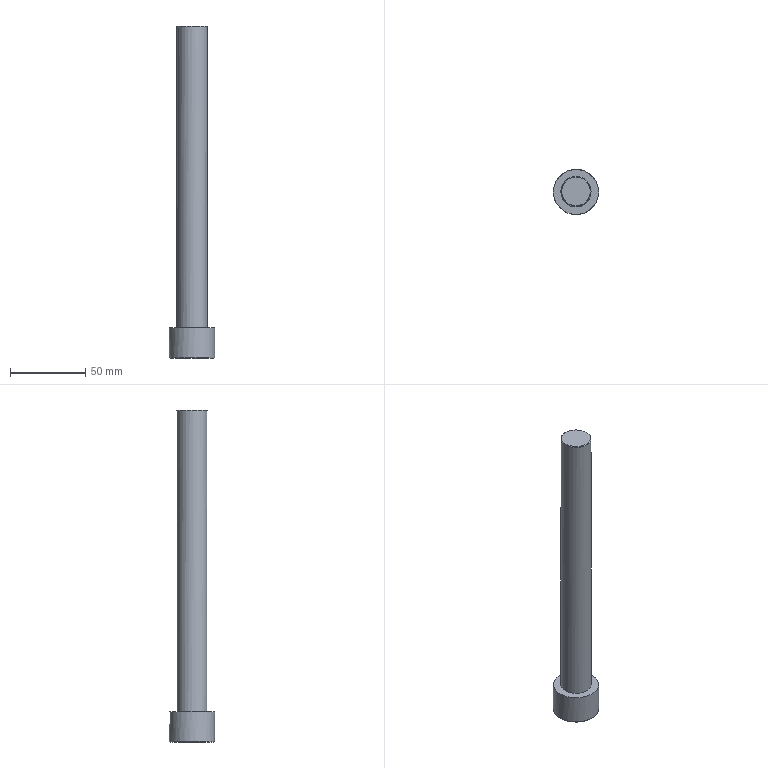Part | NX | features 模具.stp<1>[29] 2 | 1 solid | 14 faces | box 30 x 30 x 220 mm | volume 74453 mm3 | plane 10 | cylinder 2 | cone 1 | torus 1 | commonest cylinder face diameters 20 x1 30 x1
STEP:
#1=CARTESIAN_POINT('',(259.815,225.,-274.5));
#2=VERTEX_POINT('',#1);
#3=CARTESIAN_POINT('',(254.907,216.5,-274.5));
#4=VERTEX_POINT('',#3);
#5=CARTESIAN_POINT('',(259.815,225.,-274.5));
#6=DIRECTION('',(-0.5,-0.866,0.));
#7=VECTOR('',#6,1000.);
#8=LINE('',#5,#7);
#9=EDGE_CURVE('',#2,#4,#8,.T.);
#10=ORIENTED_EDGE('',*,*,#9,.T.);
#11=CARTESIAN_POINT('',(245.093,216.5,-274.5));
#12=VERTEX_POINT('',#11);
#13=CARTESIAN_POINT('',(254.907,216.5,-274.5));
#14=DIRECTION('',(-1.,0.,0.));
#15=VECTOR('',#14,1000.);
#16=LINE('',#13,#15);
#17=EDGE_CURVE('',#4,#12,#16,.T.);
#18=ORIENTED_EDGE('',*,*,#17,.T.);
#19=CARTESIAN_POINT('',(240.185,225.,-274.5));
#20=VERTEX_POINT('',#19);
#21=CARTESIAN_POINT('',(245.093,216.5,-274.5));
#22=DIRECTION('',(-0.5,0.866,0.));
#23=VECTOR('',#22,1000.);
#24=LINE('',#21,#23);
#25=EDGE_CURVE('',#12,#20,#24,.T.);
#26=ORIENTED_EDGE('',*,*,#25,.T.);
#27=CARTESIAN_POINT('',(245.093,233.5,-274.5));
#28=VERTEX_POINT('',#27);
#29=CARTESIAN_POINT('',(240.185,225.,-274.5));
#30=DIRECTION('',(0.5,0.866,0.));
#31=VECTOR('',#30,1000.);
#32=LINE('',#29,#31);
#33=EDGE_CURVE('',#20,#28,#32,.T.);
#34=ORIENTED_EDGE('',*,*,#33,.T.);
#35=CARTESIAN_POINT('',(254.907,233.5,-274.5));
#36=VERTEX_POINT('',#35);
#37=CARTESIAN_POINT('',(245.093,233.5,-274.5));
#38=DIRECTION('',(1.,0.,0.));
#39=VECTOR('',#38,1000.);
#40=LINE('',#37,#39);
#41=EDGE_CURVE('',#28,#36,#40,.T.);
#42=ORIENTED_EDGE('',*,*,#41,.T.);
#43=CARTESIAN_POINT('',(254.907,233.5,-274.5));
#44=DIRECTION('',(0.5,-0.866,0.));
#45=VECTOR('',#44,1000.);
#46=LINE('',#43,#45);
#47=EDGE_CURVE('',#36,#2,#46,.T.);
#48=ORIENTED_EDGE('',*,*,#47,.T.);
#49=EDGE_LOOP('',(#10,#18,#26,#34,#42,#48));
#50=FACE_BOUND('',#49,.T.);
#51=CARTESIAN_POINT('',(250.,225.,-274.5));
#52=DIRECTION('',(0.,0.,1.));
#53=DIRECTION('',(0.,-1.,0.));
#54=AXIS2_PLACEMENT_3D('',#51,#52,#53);
#55=PLANE('',#54);
#56=ADVANCED_FACE('',(#50),#55,.F.);
#57=CARTESIAN_POINT('',(259.815,225.,-284.5));
#58=VERTEX_POINT('',#57);
#59=CARTESIAN_POINT('',(254.907,216.5,-284.5));
#60=VERTEX_POINT('',#59);
#61=CARTESIAN_POINT('',(259.815,225.,-284.5));
#62=DIRECTION('',(-0.5,-0.866,0.));
#63=VECTOR('',#62,1000.);
#64=LINE('',#61,#63);
#65=EDGE_CURVE('',#58,#60,#64,.T.);
#66=ORIENTED_EDGE('',*,*,#65,.T.);
#67=CARTESIAN_POINT('',(254.907,216.5,-274.5));
#68=DIRECTION('',(0.,0.,-1.));
#69=VECTOR('',#68,1000.);
#70=LINE('',#67,#69);
#71=EDGE_CURVE('',#4,#60,#70,.T.);
#72=ORIENTED_EDGE('',*,*,#71,.F.);
#73=ORIENTED_EDGE('',*,*,#9,.F.);
#74=CARTESIAN_POINT('',(259.815,225.,-274.5));
#75=DIRECTION('',(0.,0.,-1.));
#76=VECTOR('',#75,1000.);
#77=LINE('',#74,#76);
#78=EDGE_CURVE('',#2,#58,#77,.T.);
#79=ORIENTED_EDGE('',*,*,#78,.T.);
#80=EDGE_LOOP('',(#66,#72,#73,#79));
#81=FACE_BOUND('',#80,.T.);
#82=CARTESIAN_POINT('',(257.361,220.75,-279.5));
#83=DIRECTION('',(0.866,-0.5,0.));
#84=DIRECTION('',(0.,0.,-1.));
#85=AXIS2_PLACEMENT_3D('',#82,#83,#84);
#86=PLANE('',#85);
#87=ADVANCED_FACE('',(#81),#86,.F.);
#88=CARTESIAN_POINT('',(245.093,216.5,-284.5));
#89=VERTEX_POINT('',#88);
#90=CARTESIAN_POINT('',(254.907,216.5,-284.5));
#91=DIRECTION('',(-1.,0.,0.));
#92=VECTOR('',#91,1000.);
#93=LINE('',#90,#92);
#94=EDGE_CURVE('',#60,#89,#93,.T.);
#95=ORIENTED_EDGE('',*,*,#94,.T.);
#96=CARTESIAN_POINT('',(245.093,216.5,-274.5));
#97=DIRECTION('',(0.,0.,-1.));
#98=VECTOR('',#97,1000.);
#99=LINE('',#96,#98);
#100=EDGE_CURVE('',#12,#89,#99,.T.);
#101=ORIENTED_EDGE('',*,*,#100,.F.);
#102=ORIENTED_EDGE('',*,*,#17,.F.);
#103=ORIENTED_EDGE('',*,*,#71,.T.);
#104=EDGE_LOOP('',(#95,#101,#102,#103));
#105=FACE_BOUND('',#104,.T.);
#106=CARTESIAN_POINT('',(250.,216.5,-279.5));
#107=DIRECTION('',(0.,-1.,0.));
#108=DIRECTION('',(0.,0.,-1.));
#109=AXIS2_PLACEMENT_3D('',#106,#107,#108);
#110=PLANE('',#109);
#111=ADVANCED_FACE('',(#105),#110,.F.);
#112=CARTESIAN_POINT('',(240.185,225.,-284.5));
#113=VERTEX_POINT('',#112);
#114=CARTESIAN_POINT('',(245.093,216.5,-284.5));
#115=DIRECTION('',(-0.5,0.866,0.));
#116=VECTOR('',#115,1000.);
#117=LINE('',#114,#116);
#118=EDGE_CURVE('',#89,#113,#117,.T.);
#119=ORIENTED_EDGE('',*,*,#118,.T.);
#120=CARTESIAN_POINT('',(240.185,225.,-274.5));
#121=DIRECTION('',(0.,0.,-1.));
#122=VECTOR('',#121,1000.);
#123=LINE('',#120,#122);
#124=EDGE_CURVE('',#20,#113,#123,.T.);
#125=ORIENTED_EDGE('',*,*,#124,.F.);
#126=ORIENTED_EDGE('',*,*,#25,.F.);
#127=ORIENTED_EDGE('',*,*,#100,.T.);
#128=EDGE_LOOP('',(#119,#125,#126,#127));
#129=FACE_BOUND('',#128,.T.);
#130=CARTESIAN_POINT('',(242.639,220.75,-279.5));
#131=DIRECTION('',(-0.866,-0.5,0.));
#132=DIRECTION('',(-0.5,0.866,0.));
#133=AXIS2_PLACEMENT_3D('',#130,#131,#132);
#134=PLANE('',#133);
#135=ADVANCED_FACE('',(#129),#134,.F.);
#136=CARTESIAN_POINT('',(245.093,233.5,-284.5));
#137=VERTEX_POINT('',#136);
#138=CARTESIAN_POINT('',(240.185,225.,-284.5));
#139=DIRECTION('',(0.5,0.866,0.));
#140=VECTOR('',#139,1000.);
#141=LINE('',#138,#140);
#142=EDGE_CURVE('',#113,#137,#141,.T.);
#143=ORIENTED_EDGE('',*,*,#142,.T.);
#144=CARTESIAN_POINT('',(245.093,233.5,-274.5));
#145=DIRECTION('',(0.,0.,-1.));
#146=VECTOR('',#145,1000.);
#147=LINE('',#144,#146);
#148=EDGE_CURVE('',#28,#137,#147,.T.);
#149=ORIENTED_EDGE('',*,*,#148,.F.);
#150=ORIENTED_EDGE('',*,*,#33,.F.);
#151=ORIENTED_EDGE('',*,*,#124,.T.);
#152=EDGE_LOOP('',(#143,#149,#150,#151));
#153=FACE_BOUND('',#152,.T.);
#154=CARTESIAN_POINT('',(242.639,229.25,-279.5));
#155=DIRECTION('',(-0.866,0.5,0.));
#156=DIRECTION('',(0.,0.,1.));
#157=AXIS2_PLACEMENT_3D('',#154,#155,#156);
#158=PLANE('',#157);
#159=ADVANCED_FACE('',(#153),#158,.F.);
#160=CARTESIAN_POINT('',(254.907,233.5,-284.5));
#161=VERTEX_POINT('',#160);
#162=CARTESIAN_POINT('',(245.093,233.5,-284.5));
#163=DIRECTION('',(1.,0.,0.));
#164=VECTOR('',#163,1000.);
#165=LINE('',#162,#164);
#166=EDGE_CURVE('',#137,#161,#165,.T.);
#167=ORIENTED_EDGE('',*,*,#166,.T.);
#168=CARTESIAN_POINT('',(254.907,233.5,-274.5));
#169=DIRECTION('',(0.,0.,-1.));
#170=VECTOR('',#169,1000.);
#171=LINE('',#168,#170);
#172=EDGE_CURVE('',#36,#161,#171,.T.);
#173=ORIENTED_EDGE('',*,*,#172,.F.);
#174=ORIENTED_EDGE('',*,*,#41,.F.);
#175=ORIENTED_EDGE('',*,*,#148,.T.);
#176=EDGE_LOOP('',(#167,#173,#174,#175));
#177=FACE_BOUND('',#176,.T.);
#178=CARTESIAN_POINT('',(250.,233.5,-279.5));
#179=DIRECTION('',(0.,1.,0.));
#180=DIRECTION('',(0.,0.,-1.));
#181=AXIS2_PLACEMENT_3D('',#178,#179,#180);
#182=PLANE('',#181);
#183=ADVANCED_FACE('',(#177),#182,.F.);
#184=CARTESIAN_POINT('',(254.907,233.5,-284.5));
#185=DIRECTION('',(0.5,-0.866,0.));
#186=VECTOR('',#185,1000.);
#187=LINE('',#184,#186);
#188=EDGE_CURVE('',#161,#58,#187,.T.);
#189=ORIENTED_EDGE('',*,*,#188,.T.);
#190=ORIENTED_EDGE('',*,*,#78,.F.);
#191=ORIENTED_EDGE('',*,*,#47,.F.);
#192=ORIENTED_EDGE('',*,*,#172,.T.);
#193=EDGE_LOOP('',(#189,#190,#191,#192));
#194=FACE_BOUND('',#193,.T.);
#195=CARTESIAN_POINT('',(257.361,229.25,-279.5));
#196=DIRECTION('',(0.866,0.5,0.));
#197=DIRECTION('',(0.,0.,-1.));
#198=AXIS2_PLACEMENT_3D('',#195,#196,#197);
#199=PLANE('',#198);
#200=ADVANCED_FACE('',(#194),#199,.F.);
#201=CARTESIAN_POINT('',(260.,225.,-65.));
#202=VERTEX_POINT('',#201);
#203=CARTESIAN_POINT('',(250.,225.,-65.));
#204=DIRECTION('',(0.,0.,-1.));
#205=DIRECTION('',(1.,0.,0.));
#206=AXIS2_PLACEMENT_3D('',#203,#204,#205);
#207=CIRCLE('',#206,10.);
#208=EDGE_CURVE('',#202,#202,#207,.T.);
#209=ORIENTED_EDGE('',*,*,#208,.F.);
#210=EDGE_LOOP('',(#209));
#211=FACE_BOUND('',#210,.T.);
#212=CARTESIAN_POINT('',(250.,215.5,-64.5));
#213=VERTEX_POINT('',#212);
#214=CARTESIAN_POINT('',(250.,225.,-64.5));
#215=DIRECTION('',(0.,0.,1.));
#216=DIRECTION('',(0.,-1.,0.));
#217=AXIS2_PLACEMENT_3D('',#214,#215,#216);
#218=CIRCLE('',#217,9.5);
#219=EDGE_CURVE('',#213,#213,#218,.T.);
#220=ORIENTED_EDGE('',*,*,#219,.F.);
#221=EDGE_LOOP('',(#220));
#222=FACE_BOUND('',#221,.T.);
#223=CARTESIAN_POINT('',(250.,225.,-65.));
#224=DIRECTION('',(0.,0.,-1.));
#225=DIRECTION('',(-1.,0.,0.));
#226=AXIS2_PLACEMENT_3D('',#223,#224,#225);
#227=CONICAL_SURFACE('',#226,10.,0.7854);
#228=ADVANCED_FACE('',(#211,#222),#227,.T.);
#229=CARTESIAN_POINT('',(260.,225.,-264.5));
#230=VERTEX_POINT('',#229);
#231=CARTESIAN_POINT('',(250.,225.,-264.5));
#232=DIRECTION('',(0.,0.,1.));
#233=DIRECTION('',(1.,0.,0.));
#234=AXIS2_PLACEMENT_3D('',#231,#232,#233);
#235=CIRCLE('',#234,10.);
#236=EDGE_CURVE('',#230,#230,#235,.T.);
#237=ORIENTED_EDGE('',*,*,#236,.T.);
#238=EDGE_LOOP('',(#237));
#239=FACE_BOUND('',#238,.T.);
#240=ORIENTED_EDGE('',*,*,#208,.T.);
#241=EDGE_LOOP('',(#240));
#242=FACE_BOUND('',#241,.T.);
#243=CARTESIAN_POINT('',(250.,225.,-64.5));
#244=DIRECTION('',(0.,0.,-1.));
#245=DIRECTION('',(1.,0.,0.));
#246=AXIS2_PLACEMENT_3D('',#243,#244,#245);
#247=CYLINDRICAL_SURFACE('',#246,10.);
#248=ADVANCED_FACE('',(#239,#242),#247,.T.);
#249=ORIENTED_EDGE('',*,*,#219,.T.);
#250=EDGE_LOOP('',(#249));
#251=FACE_BOUND('',#250,.T.);
#252=CARTESIAN_POINT('',(250.,225.,-64.5));
#253=DIRECTION('',(0.,0.,1.));
#254=DIRECTION('',(0.,-1.,0.));
#255=AXIS2_PLACEMENT_3D('',#252,#253,#254);
#256=PLANE('',#255);
#257=ADVANCED_FACE('',(#251),#256,.T.);
#258=CARTESIAN_POINT('',(250.,240.,-284.));
#259=VERTEX_POINT('',#258);
#260=CARTESIAN_POINT('',(250.,225.,-284.));
#261=DIRECTION('',(0.,0.,1.));
#262=DIRECTION('',(0.,1.,0.));
#263=AXIS2_PLACEMENT_3D('',#260,#261,#262);
#264=CIRCLE('',#263,15.);
#265=EDGE_CURVE('',#259,#259,#264,.T.);
#266=ORIENTED_EDGE('',*,*,#265,.F.);
#267=EDGE_LOOP('',(#266));
#268=FACE_BOUND('',#267,.T.);
#269=CARTESIAN_POINT('',(250.,239.5,-284.5));
#270=VERTEX_POINT('',#269);
#271=CARTESIAN_POINT('',(250.,225.,-284.5));
#272=DIRECTION('',(0.,0.,-1.));
#273=DIRECTION('',(0.,1.,0.));
#274=AXIS2_PLACEMENT_3D('',#271,#272,#273);
#275=CIRCLE('',#274,14.5);
#276=EDGE_CURVE('',#270,#270,#275,.T.);
#277=ORIENTED_EDGE('',*,*,#276,.F.);
#278=EDGE_LOOP('',(#277));
#279=FACE_BOUND('',#278,.T.);
#280=CARTESIAN_POINT('',(250.,225.,-284.));
#281=DIRECTION('',(0.,0.,-1.));
#282=DIRECTION('',(0.,1.,0.));
#283=AXIS2_PLACEMENT_3D('',#280,#281,#282);
#284=TOROIDAL_SURFACE('',#283,14.5,0.5);
#285=ADVANCED_FACE('',(#268,#279),#284,.T.);
#286=CARTESIAN_POINT('',(265.,225.,-264.5));
#287=VERTEX_POINT('',#286);
#288=CARTESIAN_POINT('',(250.,225.,-264.5));
#289=DIRECTION('',(0.,0.,-1.));
#290=DIRECTION('',(1.,0.,0.));
#291=AXIS2_PLACEMENT_3D('',#288,#289,#290);
#292=CIRCLE('',#291,15.);
#293=EDGE_CURVE('',#287,#287,#292,.T.);
#294=ORIENTED_EDGE('',*,*,#293,.T.);
#295=EDGE_LOOP('',(#294));
#296=FACE_BOUND('',#295,.T.);
#297=ORIENTED_EDGE('',*,*,#265,.T.);
#298=EDGE_LOOP('',(#297));
#299=FACE_BOUND('',#298,.T.);
#300=CARTESIAN_POINT('',(250.,225.,-264.5));
#301=DIRECTION('',(0.,0.,-1.));
#302=DIRECTION('',(1.,0.,0.));
#303=AXIS2_PLACEMENT_3D('',#300,#301,#302);
#304=CYLINDRICAL_SURFACE('',#303,15.);
#305=ADVANCED_FACE('',(#296,#299),#304,.T.);
#306=ORIENTED_EDGE('',*,*,#293,.F.);
#307=EDGE_LOOP('',(#306));
#308=FACE_BOUND('',#307,.T.);
#309=ORIENTED_EDGE('',*,*,#236,.F.);
#310=EDGE_LOOP('',(#309));
#311=FACE_BOUND('',#310,.T.);
#312=CARTESIAN_POINT('',(250.,225.,-264.5));
#313=DIRECTION('',(0.,0.,1.));
#314=DIRECTION('',(0.,-1.,0.));
#315=AXIS2_PLACEMENT_3D('',#312,#313,#314);
#316=PLANE('',#315);
#317=ADVANCED_FACE('',(#308,#311),#316,.T.);
#318=ORIENTED_EDGE('',*,*,#276,.T.);
#319=EDGE_LOOP('',(#318));
#320=FACE_BOUND('',#319,.T.);
#321=ORIENTED_EDGE('',*,*,#188,.F.);
#322=ORIENTED_EDGE('',*,*,#166,.F.);
#323=ORIENTED_EDGE('',*,*,#142,.F.);
#324=ORIENTED_EDGE('',*,*,#118,.F.);
#325=ORIENTED_EDGE('',*,*,#94,.F.);
#326=ORIENTED_EDGE('',*,*,#65,.F.);
#327=EDGE_LOOP('',(#321,#322,#323,#324,#325,#326));
#328=FACE_BOUND('',#327,.T.);
#329=CARTESIAN_POINT('',(250.,225.,-284.5));
#330=DIRECTION('',(0.,0.,-1.));
#331=DIRECTION('',(0.,-1.,0.));
#332=AXIS2_PLACEMENT_3D('',#329,#330,#331);
#333=PLANE('',#332);
#334=ADVANCED_FACE('',(#320,#328),#333,.T.);
#335=CLOSED_SHELL('',(#56,#87,#111,#135,#159,#183,#200,#228,#248,#257,#285,#305,#317,#334));
#336=MANIFOLD_SOLID_BREP('',#335);
#337=(LENGTH_UNIT()NAMED_UNIT(*)SI_UNIT(.MILLI.,.METRE.));
#338=UNCERTAINTY_MEASURE_WITH_UNIT(LENGTH_MEASURE(0.00001),#337,'','');
#339=(NAMED_UNIT(*)PLANE_ANGLE_UNIT()SI_UNIT($,.RADIAN.));
#340=(NAMED_UNIT(*)SI_UNIT($,.STERADIAN.)SOLID_ANGLE_UNIT());
#341=(GEOMETRIC_REPRESENTATION_CONTEXT(3)GLOBAL_UNCERTAINTY_ASSIGNED_CONTEXT((#338))GLOBAL_UNIT_ASSIGNED_CONTEXT((#337,#339,#340))REPRESENTATION_CONTEXT('',''));
#342=ADVANCED_BREP_SHAPE_REPRESENTATION('',(#336),#341);